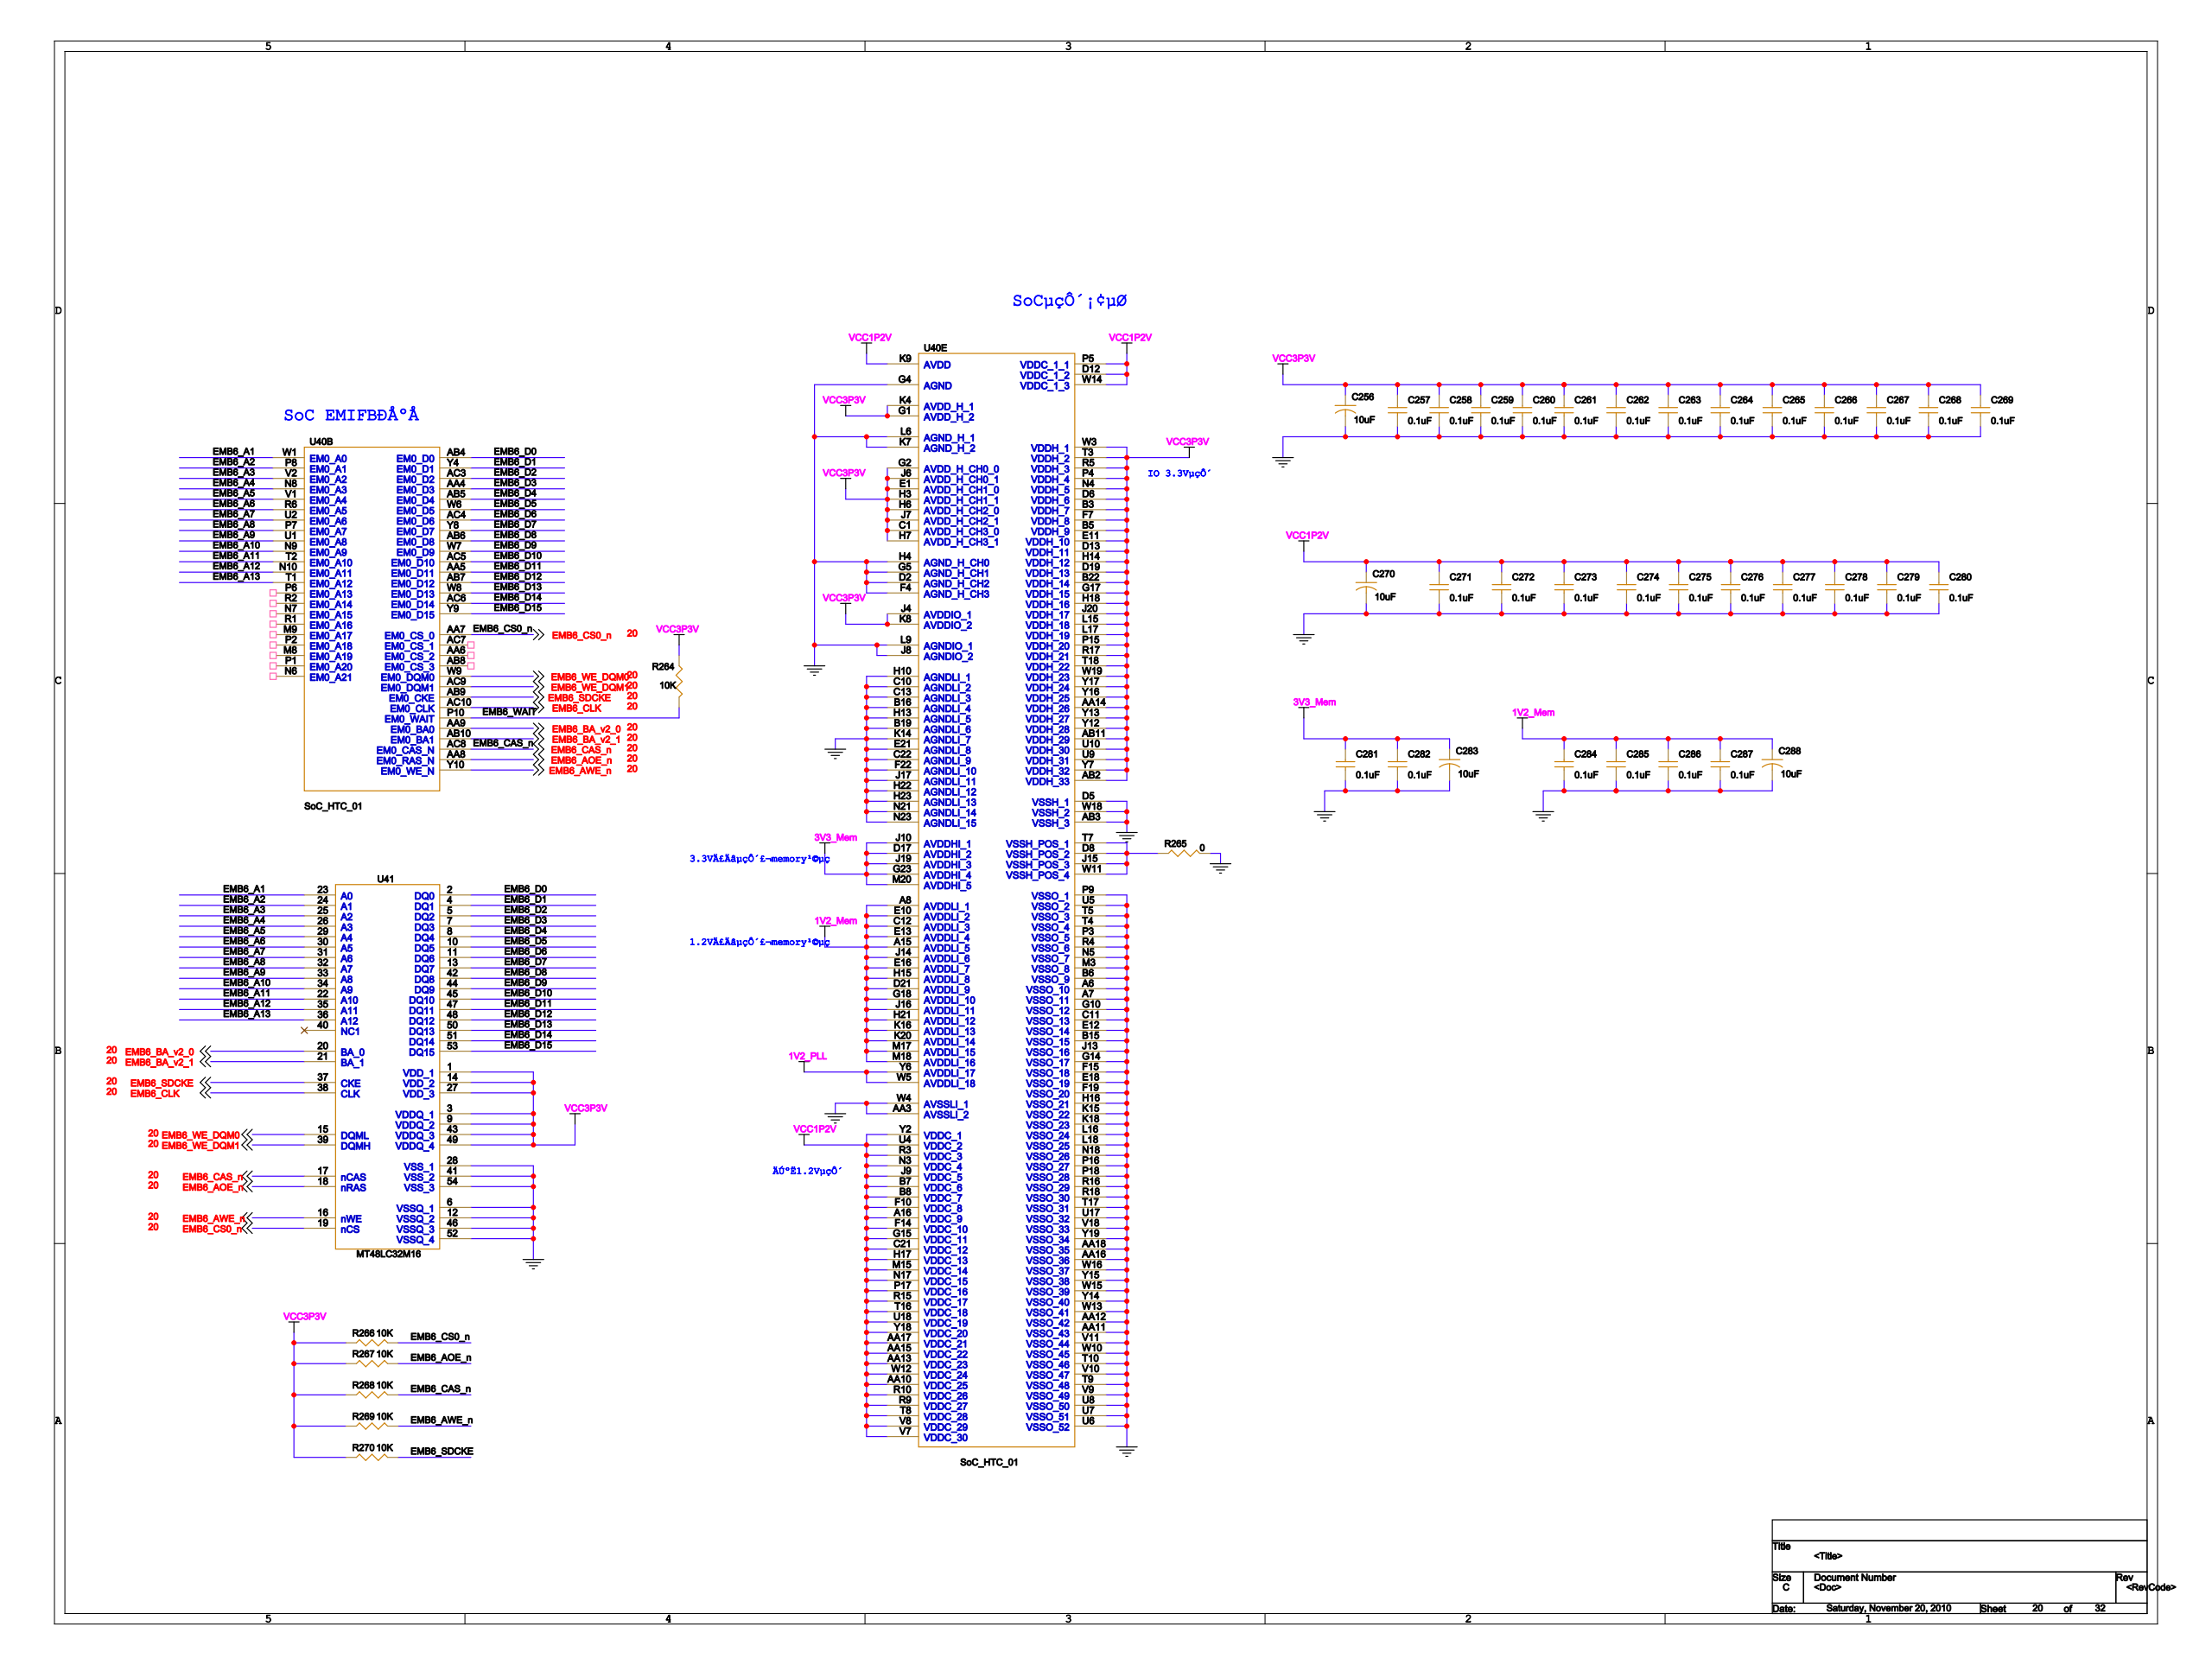Circuit board | Cadence Allegro | 1001 parts | 1318 nets | one sheet of the schematic
Parts on this sheet (reference | value | footprint):
C256 | 10uF | C3216
C257 | 0.1uF | C0402
C258 | 0.1uF | C0402
C259 | 0.1uF | C0402
C260 | 0.1uF | C0402
C261 | 0.1uF | C0402
C262 | 0.1uF | C0402
C263 | 0.1uF | C0402
C264 | 0.1uF | C0402
C265 | 0.1uF | C0402
C266 | 0.1uF | C0402
C267 | 0.1uF | C0402
C268 | 0.1uF | C0402
C269 | 0.1uF | C0402
C270 | 10uF | C3216
C271 | 0.1uF | C0402
C272 | 0.1uF | C0402
C273 | 0.1uF | C0402
C274 | 0.1uF | C0402
C275 | 0.1uF | C0402
C276 | 0.1uF | C0402
C277 | 0.1uF | C0402
C278 | 0.1uF | C0402
C279 | 0.1uF | C0402
C280 | 0.1uF | C0402
C281 | 0.1uF | C0402
C282 | 0.1uF | C0402
C283 | 10uF | C3216
C284 | 0.1uF | C0402
C285 | 0.1uF | C0402
C286 | 0.1uF | C0402
C287 | 0.1uF | C0402
C288 | 10uF | C3216
R264 | 10K | 0603
R265 | 0 | 0603
R266 | 10K | 0603
R267 | 10K | 0603
R268 | 10K | 0603
R269 | 10K | 0603
R270 | 10K | 0603
U1 | SoC_HTC_01 | L529_XIN
U2 | MT48LC32M16 | TSOP54
U4 | MAX3243 | TSSOP-28
U6 | MT48LC16M16 | TSOP54
U7 | MT48LC16M16 | TSOP54
U8 | DP83848C | DP83848C_48LQFP
U10 | SoC_HTC_01 | L529_XIN
U17 | MT48LC32M16 | TSOP54
U40 | SoC_HTC_01 | L529_XIN
U41 | MT48LC32M16 | TSOP54
Nets of these parts (net: part-pin ...):
GND: C256-2 C257-2 C258-2 C259-2 C260-2 C261-2 C262-2 C263-2 C264-2 C265-2 C266-2 C267-2 C268-2 C269-2 C270-2 C271-2 C272-2 C273-2 C274-2 C275-2 C276-2 C277-2 C278-2 C279-2 C280-2 C281-2 C282-2 C283-2 C284-2 C285-2 C286-2 C287-2 C288-2 R265-2 U1-A6 U1-A7 U1-AA3 U1-AA11 U1-AA12 U1-AA16 U1-AA18 U1-AB3 U1-B6 U1-B15 U1-B16 U1-B19 U1-C10 U1-C11 U1-C13 U1-C22 U1-D2 U1-D5 U1-E12 U1-E18 U1-E21 U1-F4 U1-F15 U1-F19 U1-F22 U1-G4 U1-G5 U1-G10 U1-G14 U1-H4 U1-H10 U1-H13 U1-H16 U1-H22 U1-H23 U1-J8 U1-J13 U1-J17 U1-K7 U1-K14 U1-K15 U1-K18 U1-L6 U1-L9 U1-L16 U1-L18 U1-M3 U1-N5 U1-N18 U1-N21 U1-N23 U1-P3 U1-P9 U1-P16 U1-P18 U1-R4 U1-R16 U1-R18 U1-T4 U1-T5 U1-T9 U1-T10 U1-T17 U1-U5 U1-U6 U1-U7 U1-U8 U1-U17 U1-V9 U1-V10 U1-V11 U1-V18 U1-W4 U1-W10 U1-W13 U1-W15 U1-W16 U1-W18 U1-Y14 U1-Y15 U1-Y19 U2-6 U2-12 U2-28 U2-41 U2-46 U2-52 U2-54 U4-23 U4-25 U6-6 U6-12 U6-28 U6-41 U6-46 U6-52 U6-54 U7-6 U7-12 U7-28 U7-41 U7-46 U7-52 U7-54 U8-15 U8-19 U8-35 U8-36 U8-47 U10-A6 U10-A7 U10-AA3 U10-AA11 U10-AA12 U10-AA16 U10-AA18 U10-AB3 U10-B6 U10-B15 U10-B16 U10-B19 U10-C10 U10-C11 U10-C13 U10-C22 U10-D2 U10-D5 U10-E12 U10-E18 U10-E21 U10-F4 U10-F15 U10-F19 U10-F22 U10-G4 U10-G5 U10-G10 U10-G14 U10-H4 U10-H10 U10-H13 U10-H16 U10-H22 U10-H23 U10-J8 U10-J13 U10-J17 U10-K7 U10-K14 U10-K15 U10-K18 U10-L6 U10-L9 U10-L16 U10-L18 U10-M3 U10-N5 U10-N18 U10-N21 U10-N23 U10-P3 U10-P9 U10-P16 U10-P18 U10-R4 U10-R16 U10-R18 U10-T4 U10-T5 U10-T9 U10-T10 U10-T17 U10-U5 U10-U6 U10-U7 U10-U8 U10-U17 U10-V9 U10-V10 U10-V11 U10-V18 U10-W4 U10-W10 U10-W13 U10-W15 U10-W16 U10-W18 U10-Y14 U10-Y15 U10-Y19 U17-6 U17-12 U17-28 U17-41 U17-46 U17-52 U17-54 U40-A6 U40-A7 U40-AA3 U40-AA11 U40-AA12 U40-AA16 U40-AA18 U40-AB3 U40-B6 U40-B15 U40-B16 U40-B19 U40-C10 U40-C11 U40-C13 U40-C22 U40-D2 U40-D5 U40-E12 U40-E18 U40-E21 U40-F4 U40-F15 U40-F19 U40-F22 U40-G4 U40-G5 U40-G10 U40-G14 U40-H4 U40-H10 U40-H13 U40-H16 U40-H22 U40-H23 U40-J8 U40-J13 U40-J17 U40-K7 U40-K14 U40-K15 U40-K18 U40-L6 U40-L9 U40-L16 U40-L18 U40-M3 U40-N5 U40-N18 U40-N21 U40-N23 U40-P3 U40-P9 U40-P16 U40-P18 U40-R4 U40-R16 U40-R18 U40-T4 U40-T5 U40-T9 U40-T10 U40-T17 U40-U5 U40-U6 U40-U7 U40-U8 U40-U17 U40-V9 U40-V10 U40-V11 U40-V18 U40-W4 U40-W10 U40-W13 U40-W15 U40-W16 U40-W18 U40-Y14 U40-Y15 U40-Y19 U41-6 U41-12 U41-28 U41-41 U41-46 U41-52 U41-54
VCC3P3V: C256-1 C257-1 C258-1 C259-1 C260-1 C261-1 C262-1 C263-1 C264-1 C265-1 C266-1 C267-1 C268-1 C269-1 R264-2 R266-1 R267-1 R268-1 R269-1 R270-1 U1-AA14 U1-AB2 U1-AB11 U1-B3 U1-B5 U1-B22 U1-C1 U1-D6 U1-D13 U1-D19 U1-E1 U1-E11 U1-F7 U1-G1 U1-G2 U1-G17 U1-H3 U1-H6 U1-H7 U1-H14 U1-H18 U1-J4 U1-J6 U1-J7 U1-J20 U1-K4 U1-K8 U1-L15 U1-L17 U1-N4 U1-P4 U1-P15 U1-R5 U1-R17 U1-T3 U1-T18 U1-U9 U1-U10 U1-W3 U1-W19 U1-Y7 U1-Y12 U1-Y13 U1-Y16 U1-Y17 U2-1 U2-3 U2-9 U2-14 U2-27 U2-43 U2-49 U4-22 U4-26 U6-1 U6-3 U6-9 U6-14 U6-27 U6-43 U6-49 U7-1 U7-3 U7-9 U7-14 U7-27 U7-43 U7-49 U8-22 U8-32 U8-48 U10-AA14 U10-AB2 U10-AB11 U10-B3 U10-B5 U10-B22 U10-C1 U10-D6 U10-D13 U10-D19 U10-E1 U10-E11 U10-F7 U10-G1 U10-G2 U10-G17 U10-H3 U10-H6 U10-H7 U10-H14 U10-H18 U10-J4 U10-J6 U10-J7 U10-J20 U10-K4 U10-K8 U10-L15 U10-L17 U10-N4 U10-P4 U10-P15 U10-R5 U10-R17 U10-T3 U10-T18 U10-U9 U10-U10 U10-W3 U10-W19 U10-Y7 U10-Y12 U10-Y13 U10-Y16 U10-Y17 U17-1 U17-3 U17-9 U17-14 U17-27 U17-43 U17-49 U40-AA14 U40-AB2 U40-AB11 U40-B3 U40-B5 U40-B22 U40-C1 U40-D6 U40-D13 U40-D19 U40-E1 U40-E11 U40-F7 U40-G1 U40-G2 U40-G17 U40-H3 U40-H6 U40-H7 U40-H14 U40-H18 U40-J4 U40-J6 U40-J7 U40-J20 U40-K4 U40-K8 U40-L15 U40-L17 U40-N4 U40-P4 U40-P15 U40-R5 U40-R17 U40-T3 U40-T18 U40-U9 U40-U10 U40-W3 U40-W19 U40-Y7 U40-Y12 U40-Y13 U40-Y16 U40-Y17 U41-1 U41-3 U41-9 U41-14 U41-27 U41-43 U41-49
VCC1P2V: C270-1 C271-1 C272-1 C273-1 C274-1 C275-1 C276-1 C277-1 C278-1 C279-1 C280-1 U1-A16 U1-AA10 U1-AA13 U1-AA15 U1-AA17 U1-B7 U1-B8 U1-C21 U1-D12 U1-F10 U1-F14 U1-G15 U1-H17 U1-J9 U1-K9 U1-M15 U1-N3 U1-N17 U1-P5 U1-P17 U1-R3 U1-R9 U1-R10 U1-R15 U1-T8 U1-T16 U1-U4 U1-U18 U1-V7 U1-V8 U1-W12 U1-W14 U1-Y2 U1-Y18 U10-A16 U10-AA10 U10-AA13 U10-AA15 U10-AA17 U10-B7 U10-B8 U10-C21 U10-D12 U10-F10 U10-F14 U10-G15 U10-H17 U10-J9 U10-K9 U10-M15 U10-N3 U10-N17 U10-P5 U10-P17 U10-R3 U10-R9 U10-R10 U10-R15 U10-T8 U10-T16 U10-U4 U10-U18 U10-V7 U10-V8 U10-W12 U10-W14 U10-Y2 U10-Y18 U40-A16 U40-AA10 U40-AA13 U40-AA15 U40-AA17 U40-B7 U40-B8 U40-C21 U40-D12 U40-F10 U40-F14 U40-G15 U40-H17 U40-J9 U40-K9 U40-M15 U40-N3 U40-N17 U40-P5 U40-P17 U40-R3 U40-R9 U40-R10 U40-R15 U40-T8 U40-T16 U40-U4 U40-U18 U40-V7 U40-V8 U40-W12 U40-W14 U40-Y2 U40-Y18
3V3_MEM: C281-1 C282-1 C283-1 U1-D17 U1-G23 U1-J10 U1-J19 U1-M20 U10-D17 U10-G23 U10-J10 U10-J19 U10-M20 U40-D17 U40-G23 U40-J10 U40-J19 U40-M20
1V2_MEM: C284-1 C285-1 C286-1 C287-1 C288-1 U1-A8 U1-A15 U1-C12 U1-D21 U1-E10 U1-E13 U1-E16 U1-G18 U1-H15 U1-H21 U1-J14 U1-J16 U1-K16 U1-K20 U1-M17 U1-M18 U10-A8 U10-A15 U10-C12 U10-D21 U10-E10 U10-E13 U10-E16 U10-G18 U10-H15 U10-H21 U10-J14 U10-J16 U10-K16 U10-K20 U10-M17 U10-M18 U40-A8 U40-A15 U40-C12 U40-D21 U40-E10 U40-E13 U40-E16 U40-G18 U40-H15 U40-H21 U40-J14 U40-J16 U40-K16 U40-K20 U40-M17 U40-M18
1V2_PLL: U1-W5 U1-Y6 U10-W5 U10-Y6 U40-W5 U40-Y6
EMB6_A1: U40-W1 U41-23
EMB6_A2: U40-P8 U41-24
EMB6_A11: U40-T2 U41-22
EMB6_A12: U40-N10 U41-35
EMB6_A13: U40-T1 U41-36
EMB6_A3: U40-V2 U41-25
EMB6_A4: U40-N8 U41-26
EMB6_A5: U40-V1 U41-29
EMB6_A6: U40-R6 U41-30
EMB6_A7: U40-U2 U41-31
EMB6_A8: U40-P7 U41-32
EMB6_A9: U40-U1 U41-33
EMB6_A10: U40-N9 U41-34
EMB6_CAS_N: R268-2 U40-AC8 U41-17
EMB6_SDCKE: R270-2 U40-AB9 U41-37
EMB6_CLK: U40-AC10 U41-38
EMB6_CS0_N: R266-2 U40-AA7 U41-19
EMB6_D0: U40-AB4 U41-2
EMB6_D1: U40-Y4 U41-4
EMB6_D10: U40-AC5 U41-45
EMB6_D11: U40-AA5 U41-47
EMB6_D12: U40-AB7 U41-48
EMB6_D13: U40-W8 U41-50
EMB6_D14: U40-AC6 U41-51
EMB6_D15: U40-Y9 U41-53
EMB6_D2: U40-AC3 U41-5
EMB6_D3: U40-AA4 U41-7
EMB6_D4: U40-AB5 U41-8
EMB6_D5: U40-W6 U41-10
EMB6_D6: U40-AC4 U41-11
EMB6_D7: U40-Y8 U41-13
EMB6_D8: U40-AB6 U41-42
EMB6_D9: U40-W7 U41-44
EMB6_WE_DQM0: U40-W9 U41-15
EMB6_WE_DQM1: U40-AC9 U41-39
EMB6_AOE_N: R267-2 U40-AA8 U41-18
EMB6_WAIT: R264-1 U40-P10
EMB6_AWE_N: R269-2 U40-Y10 U41-16
N17415091: R265-1 U40-D8 U40-J15 U40-T7 U40-W11